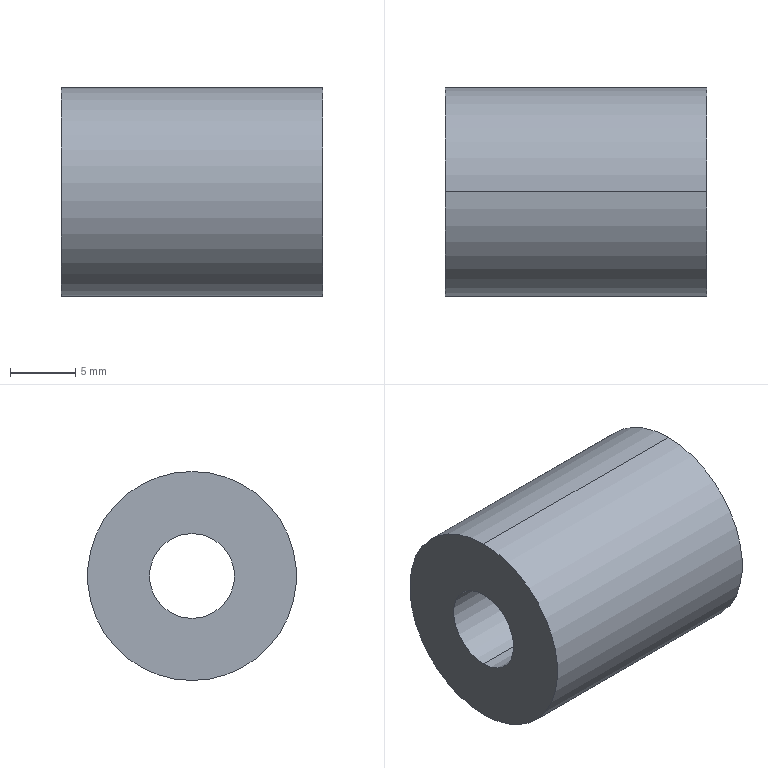Part | SolidWorks | features Extrusion 1 | 1 solid | 6 faces | box 20 x 16 x 16 mm | volume 3358 mm3 | cylinder 4 | plane 2 | commonest cylinder face diameters 6.5 x2 16 x2
STEP:
#1=CARTESIAN_POINT('',(20.,0.,3.25));
#2=VERTEX_POINT('',#1);
#3=CARTESIAN_POINT('',(20.,0.,-3.25));
#4=VERTEX_POINT('',#3);
#5=CARTESIAN_POINT('',(20.,0.,0.));
#6=DIRECTION('',(1.,0.,0.));
#7=DIRECTION('',(0.,0.,-1.));
#8=AXIS2_PLACEMENT_3D('',#5,#6,#7);
#9=CIRCLE('',#8,3.25);
#10=EDGE_CURVE('',#2,#4,#9,.T.);
#11=ORIENTED_EDGE('',*,*,#10,.T.);
#12=CARTESIAN_POINT('',(0.,0.,-3.25));
#13=VERTEX_POINT('',#12);
#14=CARTESIAN_POINT('',(20.,0.,-3.25));
#15=DIRECTION('',(-1.,0.,0.));
#16=VECTOR('',#15,1000.);
#17=LINE('',#14,#16);
#18=EDGE_CURVE('',#4,#13,#17,.T.);
#19=ORIENTED_EDGE('',*,*,#18,.T.);
#20=CARTESIAN_POINT('',(0.,0.,3.25));
#21=VERTEX_POINT('',#20);
#22=CARTESIAN_POINT('',(0.,0.,0.));
#23=DIRECTION('',(1.,0.,0.));
#24=DIRECTION('',(0.,0.,-1.));
#25=AXIS2_PLACEMENT_3D('',#22,#23,#24);
#26=CIRCLE('',#25,3.25);
#27=EDGE_CURVE('',#21,#13,#26,.T.);
#28=ORIENTED_EDGE('',*,*,#27,.F.);
#29=CARTESIAN_POINT('',(20.,0.,3.25));
#30=DIRECTION('',(-1.,0.,0.));
#31=VECTOR('',#30,1000.);
#32=LINE('',#29,#31);
#33=EDGE_CURVE('',#2,#21,#32,.T.);
#34=ORIENTED_EDGE('',*,*,#33,.F.);
#35=EDGE_LOOP('',(#11,#19,#28,#34));
#36=FACE_OUTER_BOUND('',#35,.T.);
#37=CARTESIAN_POINT('',(20.,0.,0.));
#38=DIRECTION('',(-1.,0.,0.));
#39=DIRECTION('',(0.,0.,1.));
#40=AXIS2_PLACEMENT_3D('',#37,#38,#39);
#41=CYLINDRICAL_SURFACE('',#40,3.25);
#42=ADVANCED_FACE('',(#36),#41,.F.);
#43=CARTESIAN_POINT('',(20.,0.,-8.));
#44=VERTEX_POINT('',#43);
#45=CARTESIAN_POINT('',(20.,0.,8.));
#46=VERTEX_POINT('',#45);
#47=CARTESIAN_POINT('',(20.,0.,0.));
#48=DIRECTION('',(1.,0.,0.));
#49=DIRECTION('',(0.,0.,-1.));
#50=AXIS2_PLACEMENT_3D('',#47,#48,#49);
#51=CIRCLE('',#50,8.);
#52=EDGE_CURVE('',#44,#46,#51,.T.);
#53=ORIENTED_EDGE('',*,*,#52,.F.);
#54=CARTESIAN_POINT('',(0.,0.,-8.));
#55=VERTEX_POINT('',#54);
#56=CARTESIAN_POINT('',(20.,0.,-8.));
#57=DIRECTION('',(-1.,0.,0.));
#58=VECTOR('',#57,1000.);
#59=LINE('',#56,#58);
#60=EDGE_CURVE('',#44,#55,#59,.T.);
#61=ORIENTED_EDGE('',*,*,#60,.T.);
#62=CARTESIAN_POINT('',(0.,0.,8.));
#63=VERTEX_POINT('',#62);
#64=CARTESIAN_POINT('',(0.,0.,0.));
#65=DIRECTION('',(1.,0.,0.));
#66=DIRECTION('',(0.,0.,-1.));
#67=AXIS2_PLACEMENT_3D('',#64,#65,#66);
#68=CIRCLE('',#67,8.);
#69=EDGE_CURVE('',#55,#63,#68,.T.);
#70=ORIENTED_EDGE('',*,*,#69,.T.);
#71=CARTESIAN_POINT('',(20.,0.,8.));
#72=DIRECTION('',(-1.,0.,0.));
#73=VECTOR('',#72,1000.);
#74=LINE('',#71,#73);
#75=EDGE_CURVE('',#46,#63,#74,.T.);
#76=ORIENTED_EDGE('',*,*,#75,.F.);
#77=EDGE_LOOP('',(#53,#61,#70,#76));
#78=FACE_OUTER_BOUND('',#77,.T.);
#79=CARTESIAN_POINT('',(20.,0.,0.));
#80=DIRECTION('',(-1.,0.,0.));
#81=DIRECTION('',(0.,0.,1.));
#82=AXIS2_PLACEMENT_3D('',#79,#80,#81);
#83=CYLINDRICAL_SURFACE('',#82,8.);
#84=ADVANCED_FACE('',(#78),#83,.T.);
#85=CARTESIAN_POINT('',(20.,0.,0.));
#86=DIRECTION('',(1.,0.,0.));
#87=DIRECTION('',(0.,0.,-1.));
#88=AXIS2_PLACEMENT_3D('',#85,#86,#87);
#89=CIRCLE('',#88,8.);
#90=EDGE_CURVE('',#46,#44,#89,.T.);
#91=ORIENTED_EDGE('',*,*,#90,.T.);
#92=ORIENTED_EDGE('',*,*,#52,.T.);
#93=EDGE_LOOP('',(#91,#92));
#94=FACE_OUTER_BOUND('',#93,.T.);
#95=ORIENTED_EDGE('',*,*,#10,.F.);
#96=CARTESIAN_POINT('',(20.,0.,0.));
#97=DIRECTION('',(1.,0.,0.));
#98=DIRECTION('',(0.,0.,-1.));
#99=AXIS2_PLACEMENT_3D('',#96,#97,#98);
#100=CIRCLE('',#99,3.25);
#101=EDGE_CURVE('',#4,#2,#100,.T.);
#102=ORIENTED_EDGE('',*,*,#101,.F.);
#103=EDGE_LOOP('',(#95,#102));
#104=FACE_BOUND('',#103,.T.);
#105=CARTESIAN_POINT('',(20.,0.,0.));
#106=DIRECTION('',(1.,0.,0.));
#107=DIRECTION('',(0.,0.,-1.));
#108=AXIS2_PLACEMENT_3D('',#105,#106,#107);
#109=PLANE('',#108);
#110=ADVANCED_FACE('',(#94,#104),#109,.T.);
#111=CARTESIAN_POINT('',(0.,0.,0.));
#112=DIRECTION('',(1.,0.,0.));
#113=DIRECTION('',(0.,0.,-1.));
#114=AXIS2_PLACEMENT_3D('',#111,#112,#113);
#115=CIRCLE('',#114,8.);
#116=EDGE_CURVE('',#63,#55,#115,.T.);
#117=ORIENTED_EDGE('',*,*,#116,.F.);
#118=ORIENTED_EDGE('',*,*,#69,.F.);
#119=EDGE_LOOP('',(#117,#118));
#120=FACE_OUTER_BOUND('',#119,.T.);
#121=ORIENTED_EDGE('',*,*,#27,.T.);
#122=CARTESIAN_POINT('',(0.,0.,0.));
#123=DIRECTION('',(1.,0.,0.));
#124=DIRECTION('',(0.,0.,-1.));
#125=AXIS2_PLACEMENT_3D('',#122,#123,#124);
#126=CIRCLE('',#125,3.25);
#127=EDGE_CURVE('',#13,#21,#126,.T.);
#128=ORIENTED_EDGE('',*,*,#127,.T.);
#129=EDGE_LOOP('',(#121,#128));
#130=FACE_BOUND('',#129,.T.);
#131=CARTESIAN_POINT('',(0.,0.,0.));
#132=DIRECTION('',(1.,0.,0.));
#133=DIRECTION('',(0.,0.,-1.));
#134=AXIS2_PLACEMENT_3D('',#131,#132,#133);
#135=PLANE('',#134);
#136=ADVANCED_FACE('',(#120,#130),#135,.F.);
#137=ORIENTED_EDGE('',*,*,#60,.F.);
#138=ORIENTED_EDGE('',*,*,#90,.F.);
#139=ORIENTED_EDGE('',*,*,#75,.T.);
#140=ORIENTED_EDGE('',*,*,#116,.T.);
#141=EDGE_LOOP('',(#137,#138,#139,#140));
#142=FACE_OUTER_BOUND('',#141,.T.);
#143=CARTESIAN_POINT('',(20.,0.,0.));
#144=DIRECTION('',(-1.,0.,0.));
#145=DIRECTION('',(0.,0.,1.));
#146=AXIS2_PLACEMENT_3D('',#143,#144,#145);
#147=CYLINDRICAL_SURFACE('',#146,8.);
#148=ADVANCED_FACE('',(#142),#147,.T.);
#149=ORIENTED_EDGE('',*,*,#18,.F.);
#150=ORIENTED_EDGE('',*,*,#101,.T.);
#151=ORIENTED_EDGE('',*,*,#33,.T.);
#152=ORIENTED_EDGE('',*,*,#127,.F.);
#153=EDGE_LOOP('',(#149,#150,#151,#152));
#154=FACE_OUTER_BOUND('',#153,.T.);
#155=CARTESIAN_POINT('',(20.,0.,0.));
#156=DIRECTION('',(-1.,0.,0.));
#157=DIRECTION('',(0.,0.,1.));
#158=AXIS2_PLACEMENT_3D('',#155,#156,#157);
#159=CYLINDRICAL_SURFACE('',#158,3.25);
#160=ADVANCED_FACE('',(#154),#159,.F.);
#161=CLOSED_SHELL('',(#42,#84,#110,#136,#148,#160));
#162=MANIFOLD_SOLID_BREP('',#161);
#163=CARTESIAN_POINT('',(0.,0.,0.));
#164=DIRECTION('',(0.,0.,1.));
#165=DIRECTION('',(1.,0.,0.));
#166=AXIS2_PLACEMENT_3D('',#163,#164,#165);
#167=(LENGTH_UNIT()NAMED_UNIT(*)SI_UNIT(.MILLI.,.METRE.));
#168=UNCERTAINTY_MEASURE_WITH_UNIT(LENGTH_MEASURE(0.00001),#167,'','');
#169=(NAMED_UNIT(*)PLANE_ANGLE_UNIT()SI_UNIT($,.RADIAN.));
#170=(NAMED_UNIT(*)SI_UNIT($,.STERADIAN.)SOLID_ANGLE_UNIT());
#171=(GEOMETRIC_REPRESENTATION_CONTEXT(3)GLOBAL_UNCERTAINTY_ASSIGNED_CONTEXT((#168))GLOBAL_UNIT_ASSIGNED_CONTEXT((#167,#169,#170))REPRESENTATION_CONTEXT('',''));
#172=ADVANCED_BREP_SHAPE_REPRESENTATION('',(#162,#166),#171);